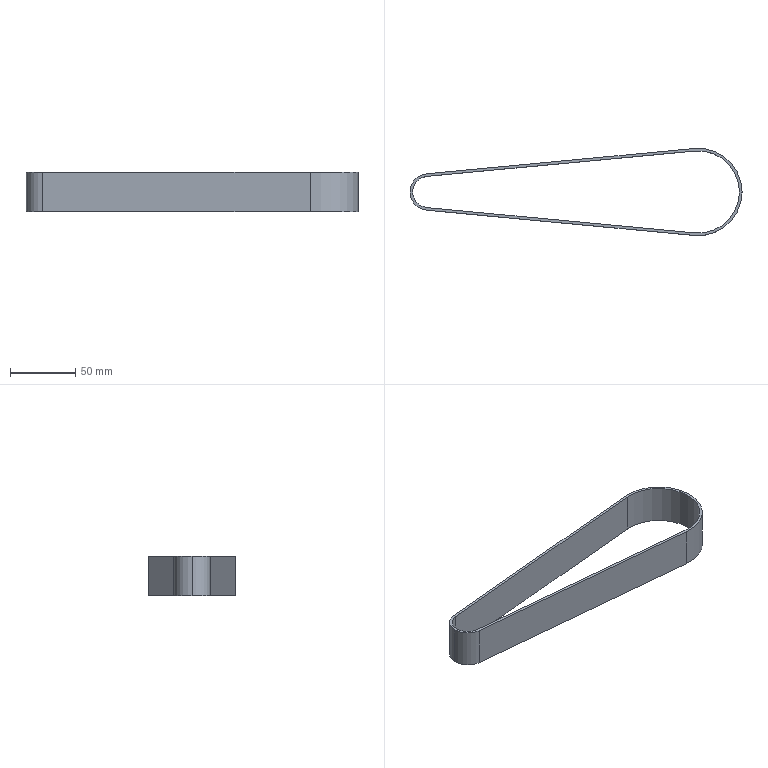Part | STEP file | Sander belt | 1 solid | 12 faces | box 254.5 x 67 x 30 mm | volume 33527 mm3 | cylinder 6 | plane 6 | commonest cylinder face diameters 24 x2 28 x2 63 x1 67 x1
STEP:
#1=CARTESIAN_POINT('',(0.,0.,0.));
#2=DIRECTION('',(0.,0.,1.));
#3=DIRECTION('',(1.,0.,0.));
#4=AXIS2_PLACEMENT_3D('',#1,#2,#3);
#5=CARTESIAN_POINT('',(-104.63,11.947,15.));
#6=VERTEX_POINT('',#5);
#7=CARTESIAN_POINT('',(-104.63,11.947,-15.));
#8=VERTEX_POINT('',#7);
#9=CARTESIAN_POINT('',(-104.63,11.947,15.));
#10=DIRECTION('',(0.,0.,-1.));
#11=VECTOR('',#10,1.);
#12=LINE('',#9,#11);
#13=CARTESIAN_POINT('',(-103.5,0.,15.));
#14=DIRECTION('',(0.,0.,-1.));
#15=DIRECTION('',(-1.,0.,0.));
#16=AXIS2_PLACEMENT_3D('',#13,#14,#15);
#17=CYLINDRICAL_SURFACE('',#16,12.);
#18=CARTESIAN_POINT('',(1.476,0.));
#19=DIRECTION('',(0.,1.));
#20=VECTOR('',#19,1.);
#21=LINE('',#18,#20);
#22=(GEOMETRIC_REPRESENTATION_CONTEXT(2)PARAMETRIC_REPRESENTATION_CONTEXT()REPRESENTATION_CONTEXT('',''));
#23=DEFINITIONAL_REPRESENTATION('',(#21),#22);
#24=PCURVE('',#17,#23);
#25=CARTESIAN_POINT('',(-104.63,11.947,15.));
#26=DIRECTION('',(0.0942,-0.9956,0.));
#27=DIRECTION('',(0.9956,0.0942,0.));
#28=AXIS2_PLACEMENT_3D('',#25,#26,#27);
#29=PLANE('',#28);
#30=CARTESIAN_POINT('',(0.,0.));
#31=DIRECTION('',(0.,-1.));
#32=VECTOR('',#31,1.);
#33=LINE('',#30,#32);
#34=(GEOMETRIC_REPRESENTATION_CONTEXT(2)PARAMETRIC_REPRESENTATION_CONTEXT()REPRESENTATION_CONTEXT('',''));
#35=DEFINITIONAL_REPRESENTATION('',(#33),#34);
#36=PCURVE('',#29,#35);
#37=SURFACE_CURVE('',#12,(#24,#36),.PCURVE_S1.);
#38=EDGE_CURVE('',#6,#8,#37,.T.);
#39=ORIENTED_EDGE('',*,*,#38,.T.);
#40=CARTESIAN_POINT('',(-115.5,0.,-15.));
#41=VERTEX_POINT('',#40);
#42=CARTESIAN_POINT('',(-103.5,0.,-15.));
#43=DIRECTION('',(0.,0.,1.));
#44=DIRECTION('',(1.,0.,0.));
#45=AXIS2_PLACEMENT_3D('',#42,#43,#44);
#46=CIRCLE('',#45,12.);
#47=CARTESIAN_POINT('',(3.142,30.));
#48=DIRECTION('',(-1.,0.));
#49=VECTOR('',#48,1.);
#50=LINE('',#47,#49);
#51=(GEOMETRIC_REPRESENTATION_CONTEXT(2)PARAMETRIC_REPRESENTATION_CONTEXT()REPRESENTATION_CONTEXT('',''));
#52=DEFINITIONAL_REPRESENTATION('',(#50),#51);
#53=PCURVE('',#17,#52);
#54=CARTESIAN_POINT('',(103.5,0.,-15.));
#55=DIRECTION('',(0.,0.,1.));
#56=DIRECTION('',(1.,0.,0.));
#57=AXIS2_PLACEMENT_3D('',#54,#55,#56);
#58=PLANE('',#57);
#59=CARTESIAN_POINT('',(-207.,0.));
#60=DIRECTION('',(1.,0.));
#61=AXIS2_PLACEMENT_2D('',#59,#60);
#62=CIRCLE('',#61,12.);
#63=(GEOMETRIC_REPRESENTATION_CONTEXT(2)PARAMETRIC_REPRESENTATION_CONTEXT()REPRESENTATION_CONTEXT('',''));
#64=DEFINITIONAL_REPRESENTATION('',(#62),#63);
#65=PCURVE('',#58,#64);
#66=SURFACE_CURVE('',#46,(#53,#65),.PCURVE_S1.);
#67=EDGE_CURVE('',#8,#41,#66,.T.);
#68=ORIENTED_EDGE('',*,*,#67,.T.);
#69=CARTESIAN_POINT('',(-115.5,0.,15.));
#70=VERTEX_POINT('',#69);
#71=CARTESIAN_POINT('',(-115.5,0.,15.));
#72=DIRECTION('',(0.,0.,-1.));
#73=VECTOR('',#72,1.);
#74=LINE('',#71,#73);
#75=CARTESIAN_POINT('',(0.,0.));
#76=DIRECTION('',(0.,1.));
#77=VECTOR('',#76,1.);
#78=LINE('',#75,#77);
#79=(GEOMETRIC_REPRESENTATION_CONTEXT(2)PARAMETRIC_REPRESENTATION_CONTEXT()REPRESENTATION_CONTEXT('',''));
#80=DEFINITIONAL_REPRESENTATION('',(#78),#79);
#81=PCURVE('',#17,#80);
#82=CARTESIAN_POINT('',(-103.5,0.,15.));
#83=DIRECTION('',(0.,0.,-1.));
#84=DIRECTION('',(-1.,0.,0.));
#85=AXIS2_PLACEMENT_3D('',#82,#83,#84);
#86=CYLINDRICAL_SURFACE('',#85,12.);
#87=CARTESIAN_POINT('',(6.283,0.));
#88=DIRECTION('',(0.,1.));
#89=VECTOR('',#88,1.);
#90=LINE('',#87,#89);
#91=(GEOMETRIC_REPRESENTATION_CONTEXT(2)PARAMETRIC_REPRESENTATION_CONTEXT()REPRESENTATION_CONTEXT('',''));
#92=DEFINITIONAL_REPRESENTATION('',(#90),#91);
#93=PCURVE('',#86,#92);
#94=SURFACE_CURVE('',#74,(#81,#93),.PCURVE_S1.);
#95=EDGE_CURVE('',#70,#41,#94,.T.);
#96=ORIENTED_EDGE('',*,*,#95,.F.);
#97=CARTESIAN_POINT('',(-103.5,0.,15.));
#98=DIRECTION('',(0.,0.,1.));
#99=DIRECTION('',(1.,0.,0.));
#100=AXIS2_PLACEMENT_3D('',#97,#98,#99);
#101=CIRCLE('',#100,12.);
#102=CARTESIAN_POINT('',(3.142,0.));
#103=DIRECTION('',(-1.,0.));
#104=VECTOR('',#103,1.);
#105=LINE('',#102,#104);
#106=(GEOMETRIC_REPRESENTATION_CONTEXT(2)PARAMETRIC_REPRESENTATION_CONTEXT()REPRESENTATION_CONTEXT('',''));
#107=DEFINITIONAL_REPRESENTATION('',(#105),#106);
#108=PCURVE('',#17,#107);
#109=CARTESIAN_POINT('',(103.5,0.,15.));
#110=DIRECTION('',(0.,0.,1.));
#111=DIRECTION('',(1.,0.,0.));
#112=AXIS2_PLACEMENT_3D('',#109,#110,#111);
#113=PLANE('',#112);
#114=CARTESIAN_POINT('',(-207.,0.));
#115=DIRECTION('',(1.,0.));
#116=AXIS2_PLACEMENT_2D('',#114,#115);
#117=CIRCLE('',#116,12.);
#118=(GEOMETRIC_REPRESENTATION_CONTEXT(2)PARAMETRIC_REPRESENTATION_CONTEXT()REPRESENTATION_CONTEXT('',''));
#119=DEFINITIONAL_REPRESENTATION('',(#117),#118);
#120=PCURVE('',#113,#119);
#121=SURFACE_CURVE('',#101,(#108,#120),.PCURVE_S1.);
#122=EDGE_CURVE('',#6,#70,#121,.T.);
#123=ORIENTED_EDGE('',*,*,#122,.F.);
#124=EDGE_LOOP('',(#39,#68,#96,#123));
#125=FACE_BOUND('',#124,.F.);
#126=ADVANCED_FACE('',(#125),#17,.F.);
#127=CARTESIAN_POINT('',(-117.5,0.,15.));
#128=VERTEX_POINT('',#127);
#129=CARTESIAN_POINT('',(-104.819,-13.938,15.));
#130=VERTEX_POINT('',#129);
#131=CARTESIAN_POINT('',(-103.5,0.,15.));
#132=DIRECTION('',(0.,0.,1.));
#133=DIRECTION('',(1.,0.,0.));
#134=AXIS2_PLACEMENT_3D('',#131,#132,#133);
#135=CIRCLE('',#134,14.);
#136=CARTESIAN_POINT('',(-103.5,0.,15.));
#137=DIRECTION('',(0.,0.,-1.));
#138=DIRECTION('',(-1.,0.,0.));
#139=AXIS2_PLACEMENT_3D('',#136,#137,#138);
#140=CYLINDRICAL_SURFACE('',#139,14.);
#141=CARTESIAN_POINT('',(9.425,0.));
#142=DIRECTION('',(-1.,0.));
#143=VECTOR('',#142,1.);
#144=LINE('',#141,#143);
#145=(GEOMETRIC_REPRESENTATION_CONTEXT(2)PARAMETRIC_REPRESENTATION_CONTEXT()REPRESENTATION_CONTEXT('',''));
#146=DEFINITIONAL_REPRESENTATION('',(#144),#145);
#147=PCURVE('',#140,#146);
#148=CARTESIAN_POINT('',(-207.,0.));
#149=DIRECTION('',(1.,0.));
#150=AXIS2_PLACEMENT_2D('',#148,#149);
#151=CIRCLE('',#150,14.);
#152=(GEOMETRIC_REPRESENTATION_CONTEXT(2)PARAMETRIC_REPRESENTATION_CONTEXT()REPRESENTATION_CONTEXT('',''));
#153=DEFINITIONAL_REPRESENTATION('',(#151),#152);
#154=PCURVE('',#113,#153);
#155=SURFACE_CURVE('',#135,(#147,#154),.PCURVE_S1.);
#156=EDGE_CURVE('',#128,#130,#155,.T.);
#157=ORIENTED_EDGE('',*,*,#156,.F.);
#158=CARTESIAN_POINT('',(-117.5,0.,-15.));
#159=VERTEX_POINT('',#158);
#160=CARTESIAN_POINT('',(-117.5,0.,15.));
#161=DIRECTION('',(0.,0.,-1.));
#162=VECTOR('',#161,1.);
#163=LINE('',#160,#162);
#164=CARTESIAN_POINT('',(6.283,0.));
#165=DIRECTION('',(0.,1.));
#166=VECTOR('',#165,1.);
#167=LINE('',#164,#166);
#168=(GEOMETRIC_REPRESENTATION_CONTEXT(2)PARAMETRIC_REPRESENTATION_CONTEXT()REPRESENTATION_CONTEXT('',''));
#169=DEFINITIONAL_REPRESENTATION('',(#167),#168);
#170=PCURVE('',#140,#169);
#171=CARTESIAN_POINT('',(-103.5,0.,15.));
#172=DIRECTION('',(0.,0.,-1.));
#173=DIRECTION('',(-1.,0.,0.));
#174=AXIS2_PLACEMENT_3D('',#171,#172,#173);
#175=CYLINDRICAL_SURFACE('',#174,14.);
#176=CARTESIAN_POINT('',(0.,0.));
#177=DIRECTION('',(0.,1.));
#178=VECTOR('',#177,1.);
#179=LINE('',#176,#178);
#180=(GEOMETRIC_REPRESENTATION_CONTEXT(2)PARAMETRIC_REPRESENTATION_CONTEXT()REPRESENTATION_CONTEXT('',''));
#181=DEFINITIONAL_REPRESENTATION('',(#179),#180);
#182=PCURVE('',#175,#181);
#183=SURFACE_CURVE('',#163,(#170,#182),.PCURVE_S1.);
#184=EDGE_CURVE('',#128,#159,#183,.T.);
#185=ORIENTED_EDGE('',*,*,#184,.T.);
#186=CARTESIAN_POINT('',(-104.819,-13.938,-15.));
#187=VERTEX_POINT('',#186);
#188=CARTESIAN_POINT('',(-103.5,0.,-15.));
#189=DIRECTION('',(0.,0.,1.));
#190=DIRECTION('',(1.,0.,0.));
#191=AXIS2_PLACEMENT_3D('',#188,#189,#190);
#192=CIRCLE('',#191,14.);
#193=CARTESIAN_POINT('',(9.425,30.));
#194=DIRECTION('',(-1.,0.));
#195=VECTOR('',#194,1.);
#196=LINE('',#193,#195);
#197=(GEOMETRIC_REPRESENTATION_CONTEXT(2)PARAMETRIC_REPRESENTATION_CONTEXT()REPRESENTATION_CONTEXT('',''));
#198=DEFINITIONAL_REPRESENTATION('',(#196),#197);
#199=PCURVE('',#140,#198);
#200=CARTESIAN_POINT('',(-207.,0.));
#201=DIRECTION('',(1.,0.));
#202=AXIS2_PLACEMENT_2D('',#200,#201);
#203=CIRCLE('',#202,14.);
#204=(GEOMETRIC_REPRESENTATION_CONTEXT(2)PARAMETRIC_REPRESENTATION_CONTEXT()REPRESENTATION_CONTEXT('',''));
#205=DEFINITIONAL_REPRESENTATION('',(#203),#204);
#206=PCURVE('',#58,#205);
#207=SURFACE_CURVE('',#192,(#199,#206),.PCURVE_S1.);
#208=EDGE_CURVE('',#159,#187,#207,.T.);
#209=ORIENTED_EDGE('',*,*,#208,.T.);
#210=CARTESIAN_POINT('',(-104.819,-13.938,15.));
#211=DIRECTION('',(0.,0.,-1.));
#212=VECTOR('',#211,1.);
#213=LINE('',#210,#212);
#214=CARTESIAN_POINT('',(4.807,0.));
#215=DIRECTION('',(0.,1.));
#216=VECTOR('',#215,1.);
#217=LINE('',#214,#216);
#218=(GEOMETRIC_REPRESENTATION_CONTEXT(2)PARAMETRIC_REPRESENTATION_CONTEXT()REPRESENTATION_CONTEXT('',''));
#219=DEFINITIONAL_REPRESENTATION('',(#217),#218);
#220=PCURVE('',#140,#219);
#221=CARTESIAN_POINT('',(-104.819,-13.938,15.));
#222=DIRECTION('',(0.0942,0.9956,0.));
#223=DIRECTION('',(-0.9956,0.0942,0.));
#224=AXIS2_PLACEMENT_3D('',#221,#222,#223);
#225=PLANE('',#224);
#226=CARTESIAN_POINT('',(0.,0.));
#227=DIRECTION('',(0.,-1.));
#228=VECTOR('',#227,1.);
#229=LINE('',#226,#228);
#230=(GEOMETRIC_REPRESENTATION_CONTEXT(2)PARAMETRIC_REPRESENTATION_CONTEXT()REPRESENTATION_CONTEXT('',''));
#231=DEFINITIONAL_REPRESENTATION('',(#229),#230);
#232=PCURVE('',#225,#231);
#233=SURFACE_CURVE('',#213,(#220,#232),.PCURVE_S1.);
#234=EDGE_CURVE('',#130,#187,#233,.T.);
#235=ORIENTED_EDGE('',*,*,#234,.F.);
#236=EDGE_LOOP('',(#157,#185,#209,#235));
#237=FACE_BOUND('',#236,.T.);
#238=ADVANCED_FACE('',(#237),#140,.T.);
#239=CARTESIAN_POINT('',(100.344,-33.351,15.));
#240=VERTEX_POINT('',#239);
#241=CARTESIAN_POINT('',(100.344,33.351,15.));
#242=VERTEX_POINT('',#241);
#243=CARTESIAN_POINT('',(103.5,0.,15.));
#244=DIRECTION('',(0.,0.,1.));
#245=DIRECTION('',(1.,0.,0.));
#246=AXIS2_PLACEMENT_3D('',#243,#244,#245);
#247=CIRCLE('',#246,33.5);
#248=CARTESIAN_POINT('',(0.,0.));
#249=DIRECTION('',(1.,0.));
#250=AXIS2_PLACEMENT_2D('',#248,#249);
#251=CIRCLE('',#250,33.5);
#252=(GEOMETRIC_REPRESENTATION_CONTEXT(2)PARAMETRIC_REPRESENTATION_CONTEXT()REPRESENTATION_CONTEXT('',''));
#253=DEFINITIONAL_REPRESENTATION('',(#251),#252);
#254=PCURVE('',#113,#253);
#255=CARTESIAN_POINT('',(103.5,0.,15.));
#256=DIRECTION('',(0.,0.,-1.));
#257=DIRECTION('',(-1.,0.,0.));
#258=AXIS2_PLACEMENT_3D('',#255,#256,#257);
#259=CYLINDRICAL_SURFACE('',#258,33.5);
#260=CARTESIAN_POINT('',(9.425,0.));
#261=DIRECTION('',(-1.,0.));
#262=VECTOR('',#261,1.);
#263=LINE('',#260,#262);
#264=(GEOMETRIC_REPRESENTATION_CONTEXT(2)PARAMETRIC_REPRESENTATION_CONTEXT()REPRESENTATION_CONTEXT('',''));
#265=DEFINITIONAL_REPRESENTATION('',(#263),#264);
#266=PCURVE('',#259,#265);
#267=SURFACE_CURVE('',#247,(#254,#266),.PCURVE_S1.);
#268=EDGE_CURVE('',#240,#242,#267,.T.);
#269=ORIENTED_EDGE('',*,*,#268,.T.);
#270=CARTESIAN_POINT('',(-104.819,13.938,15.));
#271=VERTEX_POINT('',#270);
#272=CARTESIAN_POINT('',(-104.819,13.938,15.));
#273=DIRECTION('',(-0.9956,-0.0942,0.));
#274=VECTOR('',#273,1.);
#275=LINE('',#272,#274);
#276=CARTESIAN_POINT('',(-208.319,13.938));
#277=DIRECTION('',(-0.9956,-0.0942));
#278=VECTOR('',#277,1.);
#279=LINE('',#276,#278);
#280=(GEOMETRIC_REPRESENTATION_CONTEXT(2)PARAMETRIC_REPRESENTATION_CONTEXT()REPRESENTATION_CONTEXT('',''));
#281=DEFINITIONAL_REPRESENTATION('',(#279),#280);
#282=PCURVE('',#113,#281);
#283=CARTESIAN_POINT('',(-104.819,13.938,15.));
#284=DIRECTION('',(0.0942,-0.9956,0.));
#285=DIRECTION('',(0.9956,0.0942,0.));
#286=AXIS2_PLACEMENT_3D('',#283,#284,#285);
#287=PLANE('',#286);
#288=CARTESIAN_POINT('',(0.,0.));
#289=DIRECTION('',(-1.,0.));
#290=VECTOR('',#289,1.);
#291=LINE('',#288,#290);
#292=(GEOMETRIC_REPRESENTATION_CONTEXT(2)PARAMETRIC_REPRESENTATION_CONTEXT()REPRESENTATION_CONTEXT('',''));
#293=DEFINITIONAL_REPRESENTATION('',(#291),#292);
#294=PCURVE('',#287,#293);
#295=SURFACE_CURVE('',#275,(#282,#294),.PCURVE_S1.);
#296=EDGE_CURVE('',#242,#271,#295,.T.);
#297=ORIENTED_EDGE('',*,*,#296,.T.);
#298=CARTESIAN_POINT('',(-103.5,0.,15.));
#299=DIRECTION('',(0.,0.,1.));
#300=DIRECTION('',(1.,0.,0.));
#301=AXIS2_PLACEMENT_3D('',#298,#299,#300);
#302=CIRCLE('',#301,14.);
#303=CARTESIAN_POINT('',(-207.,0.));
#304=DIRECTION('',(1.,0.));
#305=AXIS2_PLACEMENT_2D('',#303,#304);
#306=CIRCLE('',#305,14.);
#307=(GEOMETRIC_REPRESENTATION_CONTEXT(2)PARAMETRIC_REPRESENTATION_CONTEXT()REPRESENTATION_CONTEXT('',''));
#308=DEFINITIONAL_REPRESENTATION('',(#306),#307);
#309=PCURVE('',#113,#308);
#310=CARTESIAN_POINT('',(3.142,0.));
#311=DIRECTION('',(-1.,0.));
#312=VECTOR('',#311,1.);
#313=LINE('',#310,#312);
#314=(GEOMETRIC_REPRESENTATION_CONTEXT(2)PARAMETRIC_REPRESENTATION_CONTEXT()REPRESENTATION_CONTEXT('',''));
#315=DEFINITIONAL_REPRESENTATION('',(#313),#314);
#316=PCURVE('',#175,#315);
#317=SURFACE_CURVE('',#302,(#309,#316),.PCURVE_S1.);
#318=EDGE_CURVE('',#271,#128,#317,.T.);
#319=ORIENTED_EDGE('',*,*,#318,.T.);
#320=ORIENTED_EDGE('',*,*,#156,.T.);
#321=CARTESIAN_POINT('',(-104.819,-13.938,15.));
#322=DIRECTION('',(0.9956,-0.0942,0.));
#323=VECTOR('',#322,1.);
#324=LINE('',#321,#323);
#325=CARTESIAN_POINT('',(-208.319,-13.938));
#326=DIRECTION('',(0.9956,-0.0942));
#327=VECTOR('',#326,1.);
#328=LINE('',#325,#327);
#329=(GEOMETRIC_REPRESENTATION_CONTEXT(2)PARAMETRIC_REPRESENTATION_CONTEXT()REPRESENTATION_CONTEXT('',''));
#330=DEFINITIONAL_REPRESENTATION('',(#328),#329);
#331=PCURVE('',#113,#330);
#332=CARTESIAN_POINT('',(0.,0.));
#333=DIRECTION('',(-1.,0.));
#334=VECTOR('',#333,1.);
#335=LINE('',#332,#334);
#336=(GEOMETRIC_REPRESENTATION_CONTEXT(2)PARAMETRIC_REPRESENTATION_CONTEXT()REPRESENTATION_CONTEXT('',''));
#337=DEFINITIONAL_REPRESENTATION('',(#335),#336);
#338=PCURVE('',#225,#337);
#339=SURFACE_CURVE('',#324,(#331,#338),.PCURVE_S1.);
#340=EDGE_CURVE('',#130,#240,#339,.T.);
#341=ORIENTED_EDGE('',*,*,#340,.T.);
#342=EDGE_LOOP('',(#269,#297,#319,#320,#341));
#343=FACE_BOUND('',#342,.T.);
#344=CARTESIAN_POINT('',(100.533,31.36,15.));
#345=VERTEX_POINT('',#344);
#346=CARTESIAN_POINT('',(-104.63,11.947,15.));
#347=DIRECTION('',(-0.9956,-0.0942,0.));
#348=VECTOR('',#347,1.);
#349=LINE('',#346,#348);
#350=CARTESIAN_POINT('',(-208.13,11.947));
#351=DIRECTION('',(-0.9956,-0.0942));
#352=VECTOR('',#351,1.);
#353=LINE('',#350,#352);
#354=(GEOMETRIC_REPRESENTATION_CONTEXT(2)PARAMETRIC_REPRESENTATION_CONTEXT()REPRESENTATION_CONTEXT('',''));
#355=DEFINITIONAL_REPRESENTATION('',(#353),#354);
#356=PCURVE('',#113,#355);
#357=CARTESIAN_POINT('',(0.,0.));
#358=DIRECTION('',(-1.,0.));
#359=VECTOR('',#358,1.);
#360=LINE('',#357,#359);
#361=(GEOMETRIC_REPRESENTATION_CONTEXT(2)PARAMETRIC_REPRESENTATION_CONTEXT()REPRESENTATION_CONTEXT('',''));
#362=DEFINITIONAL_REPRESENTATION('',(#360),#361);
#363=PCURVE('',#29,#362);
#364=SURFACE_CURVE('',#349,(#356,#363),.PCURVE_S1.);
#365=EDGE_CURVE('',#345,#6,#364,.T.);
#366=ORIENTED_EDGE('',*,*,#365,.F.);
#367=CARTESIAN_POINT('',(100.533,-31.36,15.));
#368=VERTEX_POINT('',#367);
#369=CARTESIAN_POINT('',(103.5,0.,15.));
#370=DIRECTION('',(0.,0.,1.));
#371=DIRECTION('',(1.,0.,0.));
#372=AXIS2_PLACEMENT_3D('',#369,#370,#371);
#373=CIRCLE('',#372,31.5);
#374=CARTESIAN_POINT('',(0.,0.));
#375=DIRECTION('',(1.,0.));
#376=AXIS2_PLACEMENT_2D('',#374,#375);
#377=CIRCLE('',#376,31.5);
#378=(GEOMETRIC_REPRESENTATION_CONTEXT(2)PARAMETRIC_REPRESENTATION_CONTEXT()REPRESENTATION_CONTEXT('',''));
#379=DEFINITIONAL_REPRESENTATION('',(#377),#378);
#380=PCURVE('',#113,#379);
#381=CARTESIAN_POINT('',(103.5,0.,15.));
#382=DIRECTION('',(0.,0.,-1.));
#383=DIRECTION('',(-1.,0.,0.));
#384=AXIS2_PLACEMENT_3D('',#381,#382,#383);
#385=CYLINDRICAL_SURFACE('',#384,31.5);
#386=CARTESIAN_POINT('',(9.425,0.));
#387=DIRECTION('',(-1.,0.));
#388=VECTOR('',#387,1.);
#389=LINE('',#386,#388);
#390=(GEOMETRIC_REPRESENTATION_CONTEXT(2)PARAMETRIC_REPRESENTATION_CONTEXT()REPRESENTATION_CONTEXT('',''));
#391=DEFINITIONAL_REPRESENTATION('',(#389),#390);
#392=PCURVE('',#385,#391);
#393=SURFACE_CURVE('',#373,(#380,#392),.PCURVE_S1.);
#394=EDGE_CURVE('',#368,#345,#393,.T.);
#395=ORIENTED_EDGE('',*,*,#394,.F.);
#396=CARTESIAN_POINT('',(-104.63,-11.947,15.));
#397=VERTEX_POINT('',#396);
#398=CARTESIAN_POINT('',(-104.63,-11.947,15.));
#399=DIRECTION('',(0.9956,-0.0942,0.));
#400=VECTOR('',#399,1.);
#401=LINE('',#398,#400);
#402=CARTESIAN_POINT('',(-208.13,-11.947));
#403=DIRECTION('',(0.9956,-0.0942));
#404=VECTOR('',#403,1.);
#405=LINE('',#402,#404);
#406=(GEOMETRIC_REPRESENTATION_CONTEXT(2)PARAMETRIC_REPRESENTATION_CONTEXT()REPRESENTATION_CONTEXT('',''));
#407=DEFINITIONAL_REPRESENTATION('',(#405),#406);
#408=PCURVE('',#113,#407);
#409=CARTESIAN_POINT('',(-104.63,-11.947,15.));
#410=DIRECTION('',(0.0942,0.9956,0.));
#411=DIRECTION('',(-0.9956,0.0942,0.));
#412=AXIS2_PLACEMENT_3D('',#409,#410,#411);
#413=PLANE('',#412);
#414=CARTESIAN_POINT('',(0.,0.));
#415=DIRECTION('',(-1.,0.));
#416=VECTOR('',#415,1.);
#417=LINE('',#414,#416);
#418=(GEOMETRIC_REPRESENTATION_CONTEXT(2)PARAMETRIC_REPRESENTATION_CONTEXT()REPRESENTATION_CONTEXT('',''));
#419=DEFINITIONAL_REPRESENTATION('',(#417),#418);
#420=PCURVE('',#413,#419);
#421=SURFACE_CURVE('',#401,(#408,#420),.PCURVE_S1.);
#422=EDGE_CURVE('',#397,#368,#421,.T.);
#423=ORIENTED_EDGE('',*,*,#422,.F.);
#424=CARTESIAN_POINT('',(-103.5,0.,15.));
#425=DIRECTION('',(0.,0.,1.));
#426=DIRECTION('',(1.,0.,0.));
#427=AXIS2_PLACEMENT_3D('',#424,#425,#426);
#428=CIRCLE('',#427,12.);
#429=CARTESIAN_POINT('',(-207.,0.));
#430=DIRECTION('',(1.,0.));
#431=AXIS2_PLACEMENT_2D('',#429,#430);
#432=CIRCLE('',#431,12.);
#433=(GEOMETRIC_REPRESENTATION_CONTEXT(2)PARAMETRIC_REPRESENTATION_CONTEXT()REPRESENTATION_CONTEXT('',''));
#434=DEFINITIONAL_REPRESENTATION('',(#432),#433);
#435=PCURVE('',#113,#434);
#436=CARTESIAN_POINT('',(9.425,0.));
#437=DIRECTION('',(-1.,0.));
#438=VECTOR('',#437,1.);
#439=LINE('',#436,#438);
#440=(GEOMETRIC_REPRESENTATION_CONTEXT(2)PARAMETRIC_REPRESENTATION_CONTEXT()REPRESENTATION_CONTEXT('',''));
#441=DEFINITIONAL_REPRESENTATION('',(#439),#440);
#442=PCURVE('',#86,#441);
#443=SURFACE_CURVE('',#428,(#435,#442),.PCURVE_S1.);
#444=EDGE_CURVE('',#70,#397,#443,.T.);
#445=ORIENTED_EDGE('',*,*,#444,.F.);
#446=ORIENTED_EDGE('',*,*,#122,.F.);
#447=EDGE_LOOP('',(#366,#395,#423,#445,#446));
#448=FACE_BOUND('',#447,.T.);
#449=ADVANCED_FACE('',(#343,#448),#113,.T.);
#450=CARTESIAN_POINT('',(100.344,-33.351,-15.));
#451=VERTEX_POINT('',#450);
#452=CARTESIAN_POINT('',(100.344,33.351,-15.));
#453=VERTEX_POINT('',#452);
#454=CARTESIAN_POINT('',(103.5,0.,-15.));
#455=DIRECTION('',(0.,0.,1.));
#456=DIRECTION('',(1.,0.,0.));
#457=AXIS2_PLACEMENT_3D('',#454,#455,#456);
#458=CIRCLE('',#457,33.5);
#459=CARTESIAN_POINT('',(0.,0.));
#460=DIRECTION('',(1.,0.));
#461=AXIS2_PLACEMENT_2D('',#459,#460);
#462=CIRCLE('',#461,33.5);
#463=(GEOMETRIC_REPRESENTATION_CONTEXT(2)PARAMETRIC_REPRESENTATION_CONTEXT()REPRESENTATION_CONTEXT('',''));
#464=DEFINITIONAL_REPRESENTATION('',(#462),#463);
#465=PCURVE('',#58,#464);
#466=CARTESIAN_POINT('',(9.425,30.));
#467=DIRECTION('',(-1.,0.));
#468=VECTOR('',#467,1.);
#469=LINE('',#466,#468);
#470=(GEOMETRIC_REPRESENTATION_CONTEXT(2)PARAMETRIC_REPRESENTATION_CONTEXT()REPRESENTATION_CONTEXT('',''));
#471=DEFINITIONAL_REPRESENTATION('',(#469),#470);
#472=PCURVE('',#259,#471);
#473=SURFACE_CURVE('',#458,(#465,#472),.PCURVE_S1.);
#474=EDGE_CURVE('',#451,#453,#473,.T.);
#475=ORIENTED_EDGE('',*,*,#474,.F.);
#476=CARTESIAN_POINT('',(-104.819,-13.938,-15.));
#477=DIRECTION('',(0.9956,-0.0942,0.));
#478=VECTOR('',#477,1.);
#479=LINE('',#476,#478);
#480=CARTESIAN_POINT('',(-208.319,-13.938));
#481=DIRECTION('',(0.9956,-0.0942));
#482=VECTOR('',#481,1.);
#483=LINE('',#480,#482);
#484=(GEOMETRIC_REPRESENTATION_CONTEXT(2)PARAMETRIC_REPRESENTATION_CONTEXT()REPRESENTATION_CONTEXT('',''));
#485=DEFINITIONAL_REPRESENTATION('',(#483),#484);
#486=PCURVE('',#58,#485);
#487=CARTESIAN_POINT('',(0.,-30.));
#488=DIRECTION('',(-1.,0.));
#489=VECTOR('',#488,1.);
#490=LINE('',#487,#489);
#491=(GEOMETRIC_REPRESENTATION_CONTEXT(2)PARAMETRIC_REPRESENTATION_CONTEXT()REPRESENTATION_CONTEXT('',''));
#492=DEFINITIONAL_REPRESENTATION('',(#490),#491);
#493=PCURVE('',#225,#492);
#494=SURFACE_CURVE('',#479,(#486,#493),.PCURVE_S1.);
#495=EDGE_CURVE('',#187,#451,#494,.T.);
#496=ORIENTED_EDGE('',*,*,#495,.F.);
#497=ORIENTED_EDGE('',*,*,#208,.F.);
#498=CARTESIAN_POINT('',(-104.819,13.938,-15.));
#499=VERTEX_POINT('',#498);
#500=CARTESIAN_POINT('',(-103.5,0.,-15.));
#501=DIRECTION('',(0.,0.,1.));
#502=DIRECTION('',(1.,0.,0.));
#503=AXIS2_PLACEMENT_3D('',#500,#501,#502);
#504=CIRCLE('',#503,14.);
#505=CARTESIAN_POINT('',(-207.,0.));
#506=DIRECTION('',(1.,0.));
#507=AXIS2_PLACEMENT_2D('',#505,#506);
#508=CIRCLE('',#507,14.);
#509=(GEOMETRIC_REPRESENTATION_CONTEXT(2)PARAMETRIC_REPRESENTATION_CONTEXT()REPRESENTATION_CONTEXT('',''));
#510=DEFINITIONAL_REPRESENTATION('',(#508),#509);
#511=PCURVE('',#58,#510);
#512=CARTESIAN_POINT('',(3.142,30.));
#513=DIRECTION('',(-1.,0.));
#514=VECTOR('',#513,1.);
#515=LINE('',#512,#514);
#516=(GEOMETRIC_REPRESENTATION_CONTEXT(2)PARAMETRIC_REPRESENTATION_CONTEXT()REPRESENTATION_CONTEXT('',''));
#517=DEFINITIONAL_REPRESENTATION('',(#515),#516);
#518=PCURVE('',#175,#517);
#519=SURFACE_CURVE('',#504,(#511,#518),.PCURVE_S1.);
#520=EDGE_CURVE('',#499,#159,#519,.T.);
#521=ORIENTED_EDGE('',*,*,#520,.F.);
#522=CARTESIAN_POINT('',(-104.819,13.938,-15.));
#523=DIRECTION('',(-0.9956,-0.0942,0.));
#524=VECTOR('',#523,1.);
#525=LINE('',#522,#524);
#526=CARTESIAN_POINT('',(-208.319,13.938));
#527=DIRECTION('',(-0.9956,-0.0942));
#528=VECTOR('',#527,1.);
#529=LINE('',#526,#528);
#530=(GEOMETRIC_REPRESENTATION_CONTEXT(2)PARAMETRIC_REPRESENTATION_CONTEXT()REPRESENTATION_CONTEXT('',''));
#531=DEFINITIONAL_REPRESENTATION('',(#529),#530);
#532=PCURVE('',#58,#531);
#533=CARTESIAN_POINT('',(0.,-30.));
#534=DIRECTION('',(-1.,0.));
#535=VECTOR('',#534,1.);
#536=LINE('',#533,#535);
#537=(GEOMETRIC_REPRESENTATION_CONTEXT(2)PARAMETRIC_REPRESENTATION_CONTEXT()REPRESENTATION_CONTEXT('',''));
#538=DEFINITIONAL_REPRESENTATION('',(#536),#537);
#539=PCURVE('',#287,#538);
#540=SURFACE_CURVE('',#525,(#532,#539),.PCURVE_S1.);
#541=EDGE_CURVE('',#453,#499,#540,.T.);
#542=ORIENTED_EDGE('',*,*,#541,.F.);
#543=EDGE_LOOP('',(#475,#496,#497,#521,#542));
#544=FACE_BOUND('',#543,.T.);
#545=CARTESIAN_POINT('',(100.533,-31.36,-15.));
#546=VERTEX_POINT('',#545);
#547=CARTESIAN_POINT('',(100.533,31.36,-15.));
#548=VERTEX_POINT('',#547);
#549=CARTESIAN_POINT('',(103.5,0.,-15.));
#550=DIRECTION('',(0.,0.,1.));
#551=DIRECTION('',(1.,0.,0.));
#552=AXIS2_PLACEMENT_3D('',#549,#550,#551);
#553=CIRCLE('',#552,31.5);
#554=CARTESIAN_POINT('',(0.,0.));
#555=DIRECTION('',(1.,0.));
#556=AXIS2_PLACEMENT_2D('',#554,#555);
#557=CIRCLE('',#556,31.5);
#558=(GEOMETRIC_REPRESENTATION_CONTEXT(2)PARAMETRIC_REPRESENTATION_CONTEXT()REPRESENTATION_CONTEXT('',''));
#559=DEFINITIONAL_REPRESENTATION('',(#557),#558);
#560=PCURVE('',#58,#559);
#561=CARTESIAN_POINT('',(9.425,30.));
#562=DIRECTION('',(-1.,0.));
#563=VECTOR('',#562,1.);
#564=LINE('',#561,#563);
#565=(GEOMETRIC_REPRESENTATION_CONTEXT(2)PARAMETRIC_REPRESENTATION_CONTEXT()REPRESENTATION_CONTEXT('',''));
#566=DEFINITIONAL_REPRESENTATION('',(#564),#565);
#567=PCURVE('',#385,#566);
#568=SURFACE_CURVE('',#553,(#560,#567),.PCURVE_S1.);
#569=EDGE_CURVE('',#546,#548,#568,.T.);
#570=ORIENTED_EDGE('',*,*,#569,.T.);
#571=CARTESIAN_POINT('',(-104.63,11.947,-15.));
#572=DIRECTION('',(-0.9956,-0.0942,0.));
#573=VECTOR('',#572,1.);
#574=LINE('',#571,#573);
#575=CARTESIAN_POINT('',(-208.13,11.947));
#576=DIRECTION('',(-0.9956,-0.0942));
#577=VECTOR('',#576,1.);
#578=LINE('',#575,#577);
#579=(GEOMETRIC_REPRESENTATION_CONTEXT(2)PARAMETRIC_REPRESENTATION_CONTEXT()REPRESENTATION_CONTEXT('',''));
#580=DEFINITIONAL_REPRESENTATION('',(#578),#579);
#581=PCURVE('',#58,#580);
#582=CARTESIAN_POINT('',(0.,-30.));
#583=DIRECTION('',(-1.,0.));
#584=VECTOR('',#583,1.);
#585=LINE('',#582,#584);
#586=(GEOMETRIC_REPRESENTATION_CONTEXT(2)PARAMETRIC_REPRESENTATION_CONTEXT()REPRESENTATION_CONTEXT('',''));
#587=DEFINITIONAL_REPRESENTATION('',(#585),#586);
#588=PCURVE('',#29,#587);
#589=SURFACE_CURVE('',#574,(#581,#588),.PCURVE_S1.);
#590=EDGE_CURVE('',#548,#8,#589,.T.);
#591=ORIENTED_EDGE('',*,*,#590,.T.);
#592=ORIENTED_EDGE('',*,*,#67,.T.);
#593=CARTESIAN_POINT('',(-104.63,-11.947,-15.));
#594=VERTEX_POINT('',#593);
#595=CARTESIAN_POINT('',(-103.5,0.,-15.));
#596=DIRECTION('',(0.,0.,1.));
#597=DIRECTION('',(1.,0.,0.));
#598=AXIS2_PLACEMENT_3D('',#595,#596,#597);
#599=CIRCLE('',#598,12.);
#600=CARTESIAN_POINT('',(-207.,0.));
#601=DIRECTION('',(1.,0.));
#602=AXIS2_PLACEMENT_2D('',#600,#601);
#603=CIRCLE('',#602,12.);
#604=(GEOMETRIC_REPRESENTATION_CONTEXT(2)PARAMETRIC_REPRESENTATION_CONTEXT()REPRESENTATION_CONTEXT('',''));
#605=DEFINITIONAL_REPRESENTATION('',(#603),#604);
#606=PCURVE('',#58,#605);
#607=CARTESIAN_POINT('',(9.425,30.));
#608=DIRECTION('',(-1.,0.));
#609=VECTOR('',#608,1.);
#610=LINE('',#607,#609);
#611=(GEOMETRIC_REPRESENTATION_CONTEXT(2)PARAMETRIC_REPRESENTATION_CONTEXT()REPRESENTATION_CONTEXT('',''));
#612=DEFINITIONAL_REPRESENTATION('',(#610),#611);
#613=PCURVE('',#86,#612);
#614=SURFACE_CURVE('',#599,(#606,#613),.PCURVE_S1.);
#615=EDGE_CURVE('',#41,#594,#614,.T.);
#616=ORIENTED_EDGE('',*,*,#615,.T.);
#617=CARTESIAN_POINT('',(-104.63,-11.947,-15.));
#618=DIRECTION('',(0.9956,-0.0942,0.));
#619=VECTOR('',#618,1.);
#620=LINE('',#617,#619);
#621=CARTESIAN_POINT('',(-208.13,-11.947));
#622=DIRECTION('',(0.9956,-0.0942));
#623=VECTOR('',#622,1.);
#624=LINE('',#621,#623);
#625=(GEOMETRIC_REPRESENTATION_CONTEXT(2)PARAMETRIC_REPRESENTATION_CONTEXT()REPRESENTATION_CONTEXT('',''));
#626=DEFINITIONAL_REPRESENTATION('',(#624),#625);
#627=PCURVE('',#58,#626);
#628=CARTESIAN_POINT('',(0.,-30.));
#629=DIRECTION('',(-1.,0.));
#630=VECTOR('',#629,1.);
#631=LINE('',#628,#630);
#632=(GEOMETRIC_REPRESENTATION_CONTEXT(2)PARAMETRIC_REPRESENTATION_CONTEXT()REPRESENTATION_CONTEXT('',''));
#633=DEFINITIONAL_REPRESENTATION('',(#631),#632);
#634=PCURVE('',#413,#633);
#635=SURFACE_CURVE('',#620,(#627,#634),.PCURVE_S1.);
#636=EDGE_CURVE('',#594,#546,#635,.T.);
#637=ORIENTED_EDGE('',*,*,#636,.T.);
#638=EDGE_LOOP('',(#570,#591,#592,#616,#637));
#639=FACE_BOUND('',#638,.T.);
#640=ADVANCED_FACE('',(#544,#639),#58,.F.);
#641=ORIENTED_EDGE('',*,*,#474,.T.);
#642=CARTESIAN_POINT('',(100.344,33.351,15.));
#643=DIRECTION('',(0.,0.,-1.));
#644=VECTOR('',#643,1.);
#645=LINE('',#642,#644);
#646=CARTESIAN_POINT('',(1.476,0.));
#647=DIRECTION('',(0.,1.));
#648=VECTOR('',#647,1.);
#649=LINE('',#646,#648);
#650=(GEOMETRIC_REPRESENTATION_CONTEXT(2)PARAMETRIC_REPRESENTATION_CONTEXT()REPRESENTATION_CONTEXT('',''));
#651=DEFINITIONAL_REPRESENTATION('',(#649),#650);
#652=PCURVE('',#259,#651);
#653=CARTESIAN_POINT('',(206.079,0.));
#654=DIRECTION('',(0.,-1.));
#655=VECTOR('',#654,1.);
#656=LINE('',#653,#655);
#657=(GEOMETRIC_REPRESENTATION_CONTEXT(2)PARAMETRIC_REPRESENTATION_CONTEXT()REPRESENTATION_CONTEXT('',''));
#658=DEFINITIONAL_REPRESENTATION('',(#656),#657);
#659=PCURVE('',#287,#658);
#660=SURFACE_CURVE('',#645,(#652,#659),.PCURVE_S1.);
#661=EDGE_CURVE('',#242,#453,#660,.T.);
#662=ORIENTED_EDGE('',*,*,#661,.F.);
#663=ORIENTED_EDGE('',*,*,#268,.F.);
#664=CARTESIAN_POINT('',(100.344,-33.351,15.));
#665=DIRECTION('',(0.,0.,-1.));
#666=VECTOR('',#665,1.);
#667=LINE('',#664,#666);
#668=CARTESIAN_POINT('',(4.807,0.));
#669=DIRECTION('',(0.,1.));
#670=VECTOR('',#669,1.);
#671=LINE('',#668,#670);
#672=(GEOMETRIC_REPRESENTATION_CONTEXT(2)PARAMETRIC_REPRESENTATION_CONTEXT()REPRESENTATION_CONTEXT('',''));
#673=DEFINITIONAL_REPRESENTATION('',(#671),#672);
#674=PCURVE('',#259,#673);
#675=CARTESIAN_POINT('',(-206.079,0.));
#676=DIRECTION('',(0.,-1.));
#677=VECTOR('',#676,1.);
#678=LINE('',#675,#677);
#679=(GEOMETRIC_REPRESENTATION_CONTEXT(2)PARAMETRIC_REPRESENTATION_CONTEXT()REPRESENTATION_CONTEXT('',''));
#680=DEFINITIONAL_REPRESENTATION('',(#678),#679);
#681=PCURVE('',#225,#680);
#682=SURFACE_CURVE('',#667,(#674,#681),.PCURVE_S1.);
#683=EDGE_CURVE('',#240,#451,#682,.T.);
#684=ORIENTED_EDGE('',*,*,#683,.T.);
#685=EDGE_LOOP('',(#641,#662,#663,#684));
#686=FACE_BOUND('',#685,.T.);
#687=ADVANCED_FACE('',(#686),#259,.T.);
#688=ORIENTED_EDGE('',*,*,#541,.T.);
#689=CARTESIAN_POINT('',(-104.819,13.938,15.));
#690=DIRECTION('',(0.,0.,-1.));
#691=VECTOR('',#690,1.);
#692=LINE('',#689,#691);
#693=CARTESIAN_POINT('',(0.,0.));
#694=DIRECTION('',(0.,-1.));
#695=VECTOR('',#694,1.);
#696=LINE('',#693,#695);
#697=(GEOMETRIC_REPRESENTATION_CONTEXT(2)PARAMETRIC_REPRESENTATION_CONTEXT()REPRESENTATION_CONTEXT('',''));
#698=DEFINITIONAL_REPRESENTATION('',(#696),#697);
#699=PCURVE('',#287,#698);
#700=CARTESIAN_POINT('',(1.476,0.));
#701=DIRECTION('',(0.,1.));
#702=VECTOR('',#701,1.);
#703=LINE('',#700,#702);
#704=(GEOMETRIC_REPRESENTATION_CONTEXT(2)PARAMETRIC_REPRESENTATION_CONTEXT()REPRESENTATION_CONTEXT('',''));
#705=DEFINITIONAL_REPRESENTATION('',(#703),#704);
#706=PCURVE('',#175,#705);
#707=SURFACE_CURVE('',#692,(#699,#706),.PCURVE_S1.);
#708=EDGE_CURVE('',#271,#499,#707,.T.);
#709=ORIENTED_EDGE('',*,*,#708,.F.);
#710=ORIENTED_EDGE('',*,*,#296,.F.);
#711=ORIENTED_EDGE('',*,*,#661,.T.);
#712=EDGE_LOOP('',(#688,#709,#710,#711));
#713=FACE_BOUND('',#712,.T.);
#714=ADVANCED_FACE('',(#713),#287,.F.);
#715=ORIENTED_EDGE('',*,*,#184,.F.);
#716=ORIENTED_EDGE('',*,*,#318,.F.);
#717=ORIENTED_EDGE('',*,*,#708,.T.);
#718=ORIENTED_EDGE('',*,*,#520,.T.);
#719=EDGE_LOOP('',(#715,#716,#717,#718));
#720=FACE_BOUND('',#719,.T.);
#721=ADVANCED_FACE('',(#720),#175,.T.);
#722=ORIENTED_EDGE('',*,*,#495,.T.);
#723=ORIENTED_EDGE('',*,*,#683,.F.);
#724=ORIENTED_EDGE('',*,*,#340,.F.);
#725=ORIENTED_EDGE('',*,*,#234,.T.);
#726=EDGE_LOOP('',(#722,#723,#724,#725));
#727=FACE_BOUND('',#726,.T.);
#728=ADVANCED_FACE('',(#727),#225,.F.);
#729=CARTESIAN_POINT('',(100.533,31.36,15.));
#730=DIRECTION('',(0.,0.,-1.));
#731=VECTOR('',#730,1.);
#732=LINE('',#729,#731);
#733=CARTESIAN_POINT('',(1.476,0.));
#734=DIRECTION('',(0.,1.));
#735=VECTOR('',#734,1.);
#736=LINE('',#733,#735);
#737=(GEOMETRIC_REPRESENTATION_CONTEXT(2)PARAMETRIC_REPRESENTATION_CONTEXT()REPRESENTATION_CONTEXT('',''));
#738=DEFINITIONAL_REPRESENTATION('',(#736),#737);
#739=PCURVE('',#385,#738);
#740=CARTESIAN_POINT('',(206.079,0.));
#741=DIRECTION('',(0.,-1.));
#742=VECTOR('',#741,1.);
#743=LINE('',#740,#742);
#744=(GEOMETRIC_REPRESENTATION_CONTEXT(2)PARAMETRIC_REPRESENTATION_CONTEXT()REPRESENTATION_CONTEXT('',''));
#745=DEFINITIONAL_REPRESENTATION('',(#743),#744);
#746=PCURVE('',#29,#745);
#747=SURFACE_CURVE('',#732,(#739,#746),.PCURVE_S1.);
#748=EDGE_CURVE('',#345,#548,#747,.T.);
#749=ORIENTED_EDGE('',*,*,#748,.F.);
#750=ORIENTED_EDGE('',*,*,#394,.F.);
#751=CARTESIAN_POINT('',(100.533,-31.36,15.));
#752=DIRECTION('',(0.,0.,-1.));
#753=VECTOR('',#752,1.);
#754=LINE('',#751,#753);
#755=CARTESIAN_POINT('',(4.807,0.));
#756=DIRECTION('',(0.,1.));
#757=VECTOR('',#756,1.);
#758=LINE('',#755,#757);
#759=(GEOMETRIC_REPRESENTATION_CONTEXT(2)PARAMETRIC_REPRESENTATION_CONTEXT()REPRESENTATION_CONTEXT('',''));
#760=DEFINITIONAL_REPRESENTATION('',(#758),#759);
#761=PCURVE('',#385,#760);
#762=CARTESIAN_POINT('',(-206.079,0.));
#763=DIRECTION('',(0.,-1.));
#764=VECTOR('',#763,1.);
#765=LINE('',#762,#764);
#766=(GEOMETRIC_REPRESENTATION_CONTEXT(2)PARAMETRIC_REPRESENTATION_CONTEXT()REPRESENTATION_CONTEXT('',''));
#767=DEFINITIONAL_REPRESENTATION('',(#765),#766);
#768=PCURVE('',#413,#767);
#769=SURFACE_CURVE('',#754,(#761,#768),.PCURVE_S1.);
#770=EDGE_CURVE('',#368,#546,#769,.T.);
#771=ORIENTED_EDGE('',*,*,#770,.T.);
#772=ORIENTED_EDGE('',*,*,#569,.T.);
#773=EDGE_LOOP('',(#749,#750,#771,#772));
#774=FACE_BOUND('',#773,.F.);
#775=ADVANCED_FACE('',(#774),#385,.F.);
#776=ORIENTED_EDGE('',*,*,#590,.F.);
#777=ORIENTED_EDGE('',*,*,#748,.F.);
#778=ORIENTED_EDGE('',*,*,#365,.T.);
#779=ORIENTED_EDGE('',*,*,#38,.T.);
#780=EDGE_LOOP('',(#776,#777,#778,#779));
#781=FACE_BOUND('',#780,.T.);
#782=ADVANCED_FACE('',(#781),#29,.T.);
#783=ORIENTED_EDGE('',*,*,#615,.T.);
#784=CARTESIAN_POINT('',(-104.63,-11.947,15.));
#785=DIRECTION('',(0.,0.,-1.));
#786=VECTOR('',#785,1.);
#787=LINE('',#784,#786);
#788=CARTESIAN_POINT('',(4.807,0.));
#789=DIRECTION('',(0.,1.));
#790=VECTOR('',#789,1.);
#791=LINE('',#788,#790);
#792=(GEOMETRIC_REPRESENTATION_CONTEXT(2)PARAMETRIC_REPRESENTATION_CONTEXT()REPRESENTATION_CONTEXT('',''));
#793=DEFINITIONAL_REPRESENTATION('',(#791),#792);
#794=PCURVE('',#86,#793);
#795=CARTESIAN_POINT('',(0.,0.));
#796=DIRECTION('',(0.,-1.));
#797=VECTOR('',#796,1.);
#798=LINE('',#795,#797);
#799=(GEOMETRIC_REPRESENTATION_CONTEXT(2)PARAMETRIC_REPRESENTATION_CONTEXT()REPRESENTATION_CONTEXT('',''));
#800=DEFINITIONAL_REPRESENTATION('',(#798),#799);
#801=PCURVE('',#413,#800);
#802=SURFACE_CURVE('',#787,(#794,#801),.PCURVE_S1.);
#803=EDGE_CURVE('',#397,#594,#802,.T.);
#804=ORIENTED_EDGE('',*,*,#803,.F.);
#805=ORIENTED_EDGE('',*,*,#444,.F.);
#806=ORIENTED_EDGE('',*,*,#95,.T.);
#807=EDGE_LOOP('',(#783,#804,#805,#806));
#808=FACE_BOUND('',#807,.F.);
#809=ADVANCED_FACE('',(#808),#86,.F.);
#810=ORIENTED_EDGE('',*,*,#636,.F.);
#811=ORIENTED_EDGE('',*,*,#803,.F.);
#812=ORIENTED_EDGE('',*,*,#422,.T.);
#813=ORIENTED_EDGE('',*,*,#770,.T.);
#814=EDGE_LOOP('',(#810,#811,#812,#813));
#815=FACE_BOUND('',#814,.T.);
#816=ADVANCED_FACE('',(#815),#413,.T.);
#817=CLOSED_SHELL('',(#126,#238,#449,#640,#687,#714,#721,#728,#775,#782,#809,#816));
#818=MANIFOLD_SOLID_BREP('',#817);
#819=(LENGTH_UNIT()NAMED_UNIT(*)SI_UNIT(.MILLI.,.METRE.));
#820=UNCERTAINTY_MEASURE_WITH_UNIT(LENGTH_MEASURE(0.0000001),#819,'','');
#821=(NAMED_UNIT(*)PLANE_ANGLE_UNIT()SI_UNIT($,.RADIAN.));
#822=(NAMED_UNIT(*)SI_UNIT($,.STERADIAN.)SOLID_ANGLE_UNIT());
#823=(GEOMETRIC_REPRESENTATION_CONTEXT(3)GLOBAL_UNCERTAINTY_ASSIGNED_CONTEXT((#820))GLOBAL_UNIT_ASSIGNED_CONTEXT((#819,#821,#822))REPRESENTATION_CONTEXT('',''));
#824=ADVANCED_BREP_SHAPE_REPRESENTATION('',(#4,#818),#823);